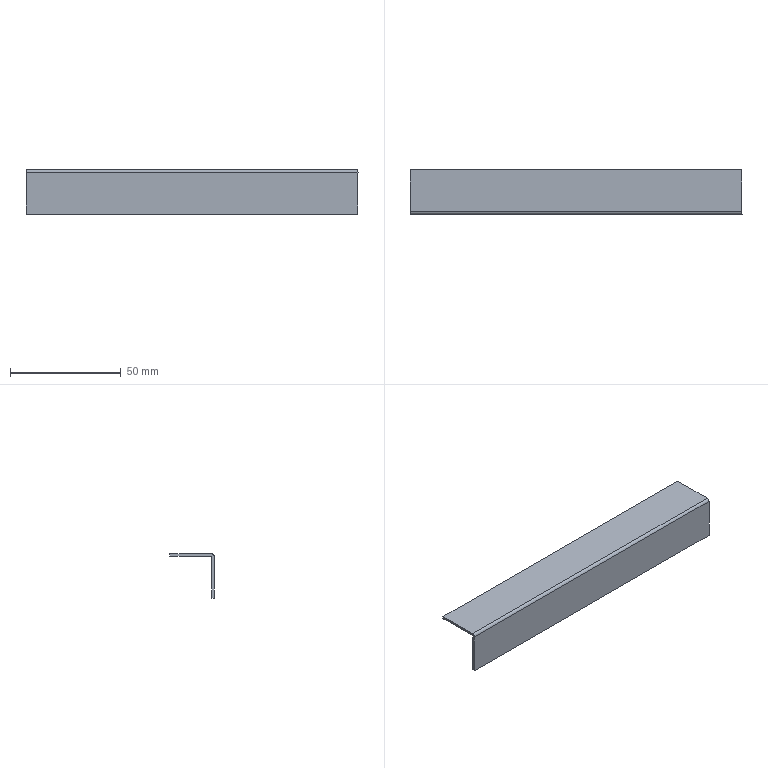Part | NX | features BREP 1 | 1 solid | 10 faces | box 150 x 20 x 20 mm | volume 5805 mm3 | plane 8 | cylinder 2 | commonest cylinder face diameters 0.4 x1 2.4 x1
STEP:
#1=CARTESIAN_POINT('',(40.,257.335,1569.));
#2=VERTEX_POINT('',#1);
#3=CARTESIAN_POINT('',(-110.,257.335,1569.));
#4=VERTEX_POINT('',#3);
#5=CARTESIAN_POINT('',(-110.,257.335,1569.));
#6=DIRECTION('',(-1.,0.,0.));
#7=VECTOR('',#6,1000.);
#8=LINE('',#5,#7);
#9=EDGE_CURVE('',#2,#4,#8,.T.);
#10=ORIENTED_EDGE('',*,*,#9,.F.);
#11=CARTESIAN_POINT('',(40.,238.535,1569.));
#12=VERTEX_POINT('',#11);
#13=CARTESIAN_POINT('',(40.,238.335,1569.));
#14=DIRECTION('',(0.,1.,0.));
#15=VECTOR('',#14,1000.);
#16=LINE('',#13,#15);
#17=EDGE_CURVE('',#12,#2,#16,.T.);
#18=ORIENTED_EDGE('',*,*,#17,.F.);
#19=CARTESIAN_POINT('',(-110.,238.535,1569.));
#20=VERTEX_POINT('',#19);
#21=CARTESIAN_POINT('',(-110.,238.535,1569.));
#22=DIRECTION('',(1.,0.,0.));
#23=VECTOR('',#22,1000.);
#24=LINE('',#21,#23);
#25=EDGE_CURVE('',#20,#12,#24,.T.);
#26=ORIENTED_EDGE('',*,*,#25,.F.);
#27=CARTESIAN_POINT('',(-110.,238.335,1569.));
#28=DIRECTION('',(0.,-1.,0.));
#29=VECTOR('',#28,1000.);
#30=LINE('',#27,#29);
#31=EDGE_CURVE('',#4,#20,#30,.T.);
#32=ORIENTED_EDGE('',*,*,#31,.F.);
#33=EDGE_LOOP('',(#10,#18,#26,#32));
#34=FACE_BOUND('',#33,.T.);
#35=CARTESIAN_POINT('',(-110.,238.335,1569.));
#36=DIRECTION('',(0.,0.,1.));
#37=DIRECTION('',(0.,1.,0.));
#38=AXIS2_PLACEMENT_3D('',#35,#36,#37);
#39=PLANE('',#38);
#40=ADVANCED_FACE('',(#34),#39,.F.);
#41=CARTESIAN_POINT('',(-110.,237.335,1568.8));
#42=VERTEX_POINT('',#41);
#43=CARTESIAN_POINT('',(-110.,237.335,1550.));
#44=VERTEX_POINT('',#43);
#45=CARTESIAN_POINT('',(-110.,237.335,1550.));
#46=DIRECTION('',(0.,0.,-1.));
#47=VECTOR('',#46,1000.);
#48=LINE('',#45,#47);
#49=EDGE_CURVE('',#42,#44,#48,.T.);
#50=ORIENTED_EDGE('',*,*,#49,.F.);
#51=CARTESIAN_POINT('',(-110.,238.535,1570.));
#52=VERTEX_POINT('',#51);
#53=CARTESIAN_POINT('',(-110.,238.535,1568.8));
#54=DIRECTION('',(1.,0.,0.));
#55=DIRECTION('',(0.,-1.,0.));
#56=AXIS2_PLACEMENT_3D('',#53,#54,#55);
#57=CIRCLE('',#56,1.2);
#58=EDGE_CURVE('',#52,#42,#57,.T.);
#59=ORIENTED_EDGE('',*,*,#58,.F.);
#60=CARTESIAN_POINT('',(-110.,257.335,1570.));
#61=VERTEX_POINT('',#60);
#62=CARTESIAN_POINT('',(-110.,238.335,1570.));
#63=DIRECTION('',(0.,-1.,0.));
#64=VECTOR('',#63,1000.);
#65=LINE('',#62,#64);
#66=EDGE_CURVE('',#61,#52,#65,.T.);
#67=ORIENTED_EDGE('',*,*,#66,.F.);
#68=CARTESIAN_POINT('',(-110.,257.335,1550.));
#69=DIRECTION('',(0.,0.,1.));
#70=VECTOR('',#69,1000.);
#71=LINE('',#68,#70);
#72=EDGE_CURVE('',#4,#61,#71,.T.);
#73=ORIENTED_EDGE('',*,*,#72,.F.);
#74=ORIENTED_EDGE('',*,*,#31,.T.);
#75=CARTESIAN_POINT('',(-110.,238.335,1568.8));
#76=VERTEX_POINT('',#75);
#77=CARTESIAN_POINT('',(-110.,238.535,1568.8));
#78=DIRECTION('',(-1.,0.,0.));
#79=DIRECTION('',(0.,1.,0.));
#80=AXIS2_PLACEMENT_3D('',#77,#78,#79);
#81=CIRCLE('',#80,0.2);
#82=EDGE_CURVE('',#76,#20,#81,.T.);
#83=ORIENTED_EDGE('',*,*,#82,.F.);
#84=CARTESIAN_POINT('',(-110.,238.335,1550.));
#85=VERTEX_POINT('',#84);
#86=CARTESIAN_POINT('',(-110.,238.335,1550.));
#87=DIRECTION('',(0.,0.,1.));
#88=VECTOR('',#87,1000.);
#89=LINE('',#86,#88);
#90=EDGE_CURVE('',#85,#76,#89,.T.);
#91=ORIENTED_EDGE('',*,*,#90,.F.);
#92=CARTESIAN_POINT('',(-110.,238.335,1550.));
#93=DIRECTION('',(0.,1.,0.));
#94=VECTOR('',#93,1000.);
#95=LINE('',#92,#94);
#96=EDGE_CURVE('',#44,#85,#95,.T.);
#97=ORIENTED_EDGE('',*,*,#96,.F.);
#98=EDGE_LOOP('',(#50,#59,#67,#73,#74,#83,#91,#97));
#99=FACE_BOUND('',#98,.T.);
#100=CARTESIAN_POINT('',(-110.,238.335,1550.));
#101=DIRECTION('',(1.,0.,0.));
#102=DIRECTION('',(0.,-1.,0.));
#103=AXIS2_PLACEMENT_3D('',#100,#101,#102);
#104=PLANE('',#103);
#105=ADVANCED_FACE('',(#99),#104,.F.);
#106=CARTESIAN_POINT('',(40.,257.335,1570.));
#107=VERTEX_POINT('',#106);
#108=CARTESIAN_POINT('',(40.,257.335,0.));
#109=DIRECTION('',(0.,0.,-1.));
#110=VECTOR('',#109,1000.);
#111=LINE('',#108,#110);
#112=EDGE_CURVE('',#107,#2,#111,.T.);
#113=ORIENTED_EDGE('',*,*,#112,.T.);
#114=ORIENTED_EDGE('',*,*,#9,.T.);
#115=ORIENTED_EDGE('',*,*,#72,.T.);
#116=CARTESIAN_POINT('',(-0.000000014,257.335,1570.));
#117=DIRECTION('',(1.,0.,0.));
#118=VECTOR('',#117,1000.);
#119=LINE('',#116,#118);
#120=EDGE_CURVE('',#61,#107,#119,.T.);
#121=ORIENTED_EDGE('',*,*,#120,.T.);
#122=EDGE_LOOP('',(#113,#114,#115,#121));
#123=FACE_BOUND('',#122,.T.);
#124=CARTESIAN_POINT('',(-0.000000014,257.335,0.));
#125=DIRECTION('',(0.,1.,0.));
#126=DIRECTION('',(1.,0.,0.));
#127=AXIS2_PLACEMENT_3D('',#124,#125,#126);
#128=PLANE('',#127);
#129=ADVANCED_FACE('',(#123),#128,.T.);
#130=CARTESIAN_POINT('',(40.,238.535,1570.));
#131=VERTEX_POINT('',#130);
#132=CARTESIAN_POINT('',(40.,238.335,1570.));
#133=DIRECTION('',(0.,1.,0.));
#134=VECTOR('',#133,1000.);
#135=LINE('',#132,#134);
#136=EDGE_CURVE('',#131,#107,#135,.T.);
#137=ORIENTED_EDGE('',*,*,#136,.F.);
#138=CARTESIAN_POINT('',(40.,237.335,1568.8));
#139=VERTEX_POINT('',#138);
#140=CARTESIAN_POINT('',(40.,238.535,1568.8));
#141=DIRECTION('',(-1.,0.,0.));
#142=DIRECTION('',(0.,-1.,0.));
#143=AXIS2_PLACEMENT_3D('',#140,#141,#142);
#144=CIRCLE('',#143,1.2);
#145=EDGE_CURVE('',#139,#131,#144,.T.);
#146=ORIENTED_EDGE('',*,*,#145,.F.);
#147=CARTESIAN_POINT('',(40.,237.335,1550.));
#148=VERTEX_POINT('',#147);
#149=CARTESIAN_POINT('',(40.,237.335,1570.));
#150=DIRECTION('',(0.,0.,1.));
#151=VECTOR('',#150,1000.);
#152=LINE('',#149,#151);
#153=EDGE_CURVE('',#148,#139,#152,.T.);
#154=ORIENTED_EDGE('',*,*,#153,.F.);
#155=CARTESIAN_POINT('',(40.,238.335,1550.));
#156=VERTEX_POINT('',#155);
#157=CARTESIAN_POINT('',(40.,238.335,1550.));
#158=DIRECTION('',(0.,-1.,0.));
#159=VECTOR('',#158,1000.);
#160=LINE('',#157,#159);
#161=EDGE_CURVE('',#156,#148,#160,.T.);
#162=ORIENTED_EDGE('',*,*,#161,.F.);
#163=CARTESIAN_POINT('',(40.,238.335,1568.8));
#164=VERTEX_POINT('',#163);
#165=CARTESIAN_POINT('',(40.,238.335,1570.));
#166=DIRECTION('',(0.,0.,-1.));
#167=VECTOR('',#166,1000.);
#168=LINE('',#165,#167);
#169=EDGE_CURVE('',#164,#156,#168,.T.);
#170=ORIENTED_EDGE('',*,*,#169,.F.);
#171=CARTESIAN_POINT('',(40.,238.535,1568.8));
#172=DIRECTION('',(1.,0.,0.));
#173=DIRECTION('',(0.,1.,0.));
#174=AXIS2_PLACEMENT_3D('',#171,#172,#173);
#175=CIRCLE('',#174,0.2);
#176=EDGE_CURVE('',#12,#164,#175,.T.);
#177=ORIENTED_EDGE('',*,*,#176,.F.);
#178=ORIENTED_EDGE('',*,*,#17,.T.);
#179=ORIENTED_EDGE('',*,*,#112,.F.);
#180=EDGE_LOOP('',(#137,#146,#154,#162,#170,#177,#178,#179));
#181=FACE_BOUND('',#180,.T.);
#182=CARTESIAN_POINT('',(40.,238.335,1570.));
#183=DIRECTION('',(-1.,0.,0.));
#184=DIRECTION('',(0.,1.,0.));
#185=AXIS2_PLACEMENT_3D('',#182,#183,#184);
#186=PLANE('',#185);
#187=ADVANCED_FACE('',(#181),#186,.F.);
#188=ORIENTED_EDGE('',*,*,#25,.T.);
#189=ORIENTED_EDGE('',*,*,#176,.T.);
#190=CARTESIAN_POINT('',(-35.,238.335,1568.8));
#191=DIRECTION('',(1.,0.,0.));
#192=VECTOR('',#191,1000.);
#193=LINE('',#190,#192);
#194=EDGE_CURVE('',#76,#164,#193,.T.);
#195=ORIENTED_EDGE('',*,*,#194,.F.);
#196=ORIENTED_EDGE('',*,*,#82,.T.);
#197=EDGE_LOOP('',(#188,#189,#195,#196));
#198=FACE_BOUND('',#197,.T.);
#199=CARTESIAN_POINT('',(-35.,238.535,1568.8));
#200=DIRECTION('',(1.,0.,0.));
#201=DIRECTION('',(0.,-1.,0.));
#202=AXIS2_PLACEMENT_3D('',#199,#200,#201);
#203=CYLINDRICAL_SURFACE('',#202,0.2);
#204=ADVANCED_FACE('',(#198),#203,.F.);
#205=ORIENTED_EDGE('',*,*,#49,.T.);
#206=CARTESIAN_POINT('',(-0.000000012,237.335,1550.));
#207=DIRECTION('',(1.,0.,0.));
#208=VECTOR('',#207,1000.);
#209=LINE('',#206,#208);
#210=EDGE_CURVE('',#44,#148,#209,.T.);
#211=ORIENTED_EDGE('',*,*,#210,.T.);
#212=ORIENTED_EDGE('',*,*,#153,.T.);
#213=CARTESIAN_POINT('',(-0.000000012,237.335,1568.8));
#214=DIRECTION('',(-1.,0.,0.));
#215=VECTOR('',#214,1000.);
#216=LINE('',#213,#215);
#217=EDGE_CURVE('',#139,#42,#216,.T.);
#218=ORIENTED_EDGE('',*,*,#217,.T.);
#219=EDGE_LOOP('',(#205,#211,#212,#218));
#220=FACE_BOUND('',#219,.T.);
#221=CARTESIAN_POINT('',(-0.000000012,237.335,0.));
#222=DIRECTION('',(0.,-1.,0.));
#223=DIRECTION('',(-1.,0.,0.));
#224=AXIS2_PLACEMENT_3D('',#221,#222,#223);
#225=PLANE('',#224);
#226=ADVANCED_FACE('',(#220),#225,.T.);
#227=ORIENTED_EDGE('',*,*,#58,.T.);
#228=ORIENTED_EDGE('',*,*,#217,.F.);
#229=ORIENTED_EDGE('',*,*,#145,.T.);
#230=CARTESIAN_POINT('',(-35.,238.535,1570.));
#231=DIRECTION('',(-1.,0.,0.));
#232=VECTOR('',#231,1000.);
#233=LINE('',#230,#232);
#234=EDGE_CURVE('',#131,#52,#233,.T.);
#235=ORIENTED_EDGE('',*,*,#234,.T.);
#236=EDGE_LOOP('',(#227,#228,#229,#235));
#237=FACE_BOUND('',#236,.T.);
#238=CARTESIAN_POINT('',(-35.,238.535,1568.8));
#239=DIRECTION('',(-1.,0.,0.));
#240=DIRECTION('',(0.,1.,0.));
#241=AXIS2_PLACEMENT_3D('',#238,#239,#240);
#242=CYLINDRICAL_SURFACE('',#241,1.2);
#243=ADVANCED_FACE('',(#237),#242,.T.);
#244=ORIENTED_EDGE('',*,*,#136,.T.);
#245=ORIENTED_EDGE('',*,*,#120,.F.);
#246=ORIENTED_EDGE('',*,*,#66,.T.);
#247=ORIENTED_EDGE('',*,*,#234,.F.);
#248=EDGE_LOOP('',(#244,#245,#246,#247));
#249=FACE_BOUND('',#248,.T.);
#250=CARTESIAN_POINT('',(40.,238.335,1570.));
#251=DIRECTION('',(0.,0.,1.));
#252=DIRECTION('',(0.,1.,0.));
#253=AXIS2_PLACEMENT_3D('',#250,#251,#252);
#254=PLANE('',#253);
#255=ADVANCED_FACE('',(#249),#254,.T.);
#256=CARTESIAN_POINT('',(-0.000000013,238.335,1550.));
#257=DIRECTION('',(1.,0.,0.));
#258=VECTOR('',#257,1000.);
#259=LINE('',#256,#258);
#260=EDGE_CURVE('',#85,#156,#259,.T.);
#261=ORIENTED_EDGE('',*,*,#260,.F.);
#262=ORIENTED_EDGE('',*,*,#90,.T.);
#263=ORIENTED_EDGE('',*,*,#194,.T.);
#264=ORIENTED_EDGE('',*,*,#169,.T.);
#265=EDGE_LOOP('',(#261,#262,#263,#264));
#266=FACE_BOUND('',#265,.T.);
#267=CARTESIAN_POINT('',(-0.000000013,238.335,0.));
#268=DIRECTION('',(0.,-1.,0.));
#269=DIRECTION('',(-1.,0.,0.));
#270=AXIS2_PLACEMENT_3D('',#267,#268,#269);
#271=PLANE('',#270);
#272=ADVANCED_FACE('',(#266),#271,.F.);
#273=ORIENTED_EDGE('',*,*,#96,.T.);
#274=ORIENTED_EDGE('',*,*,#260,.T.);
#275=ORIENTED_EDGE('',*,*,#161,.T.);
#276=ORIENTED_EDGE('',*,*,#210,.F.);
#277=EDGE_LOOP('',(#273,#274,#275,#276));
#278=FACE_BOUND('',#277,.T.);
#279=CARTESIAN_POINT('',(-110.,238.335,1550.));
#280=DIRECTION('',(0.,0.,-1.));
#281=DIRECTION('',(0.,-1.,0.));
#282=AXIS2_PLACEMENT_3D('',#279,#280,#281);
#283=PLANE('',#282);
#284=ADVANCED_FACE('',(#278),#283,.T.);
#285=CLOSED_SHELL('',(#40,#105,#129,#187,#204,#226,#243,#255,#272,#284));
#286=MANIFOLD_SOLID_BREP('',#285);
#287=(LENGTH_UNIT()NAMED_UNIT(*)SI_UNIT(.MILLI.,.METRE.));
#288=UNCERTAINTY_MEASURE_WITH_UNIT(LENGTH_MEASURE(0.00001),#287,'','');
#289=(NAMED_UNIT(*)PLANE_ANGLE_UNIT()SI_UNIT($,.RADIAN.));
#290=(NAMED_UNIT(*)SI_UNIT($,.STERADIAN.)SOLID_ANGLE_UNIT());
#291=(GEOMETRIC_REPRESENTATION_CONTEXT(3)GLOBAL_UNCERTAINTY_ASSIGNED_CONTEXT((#288))GLOBAL_UNIT_ASSIGNED_CONTEXT((#287,#289,#290))REPRESENTATION_CONTEXT('',''));
#292=ADVANCED_BREP_SHAPE_REPRESENTATION('',(#286),#291);